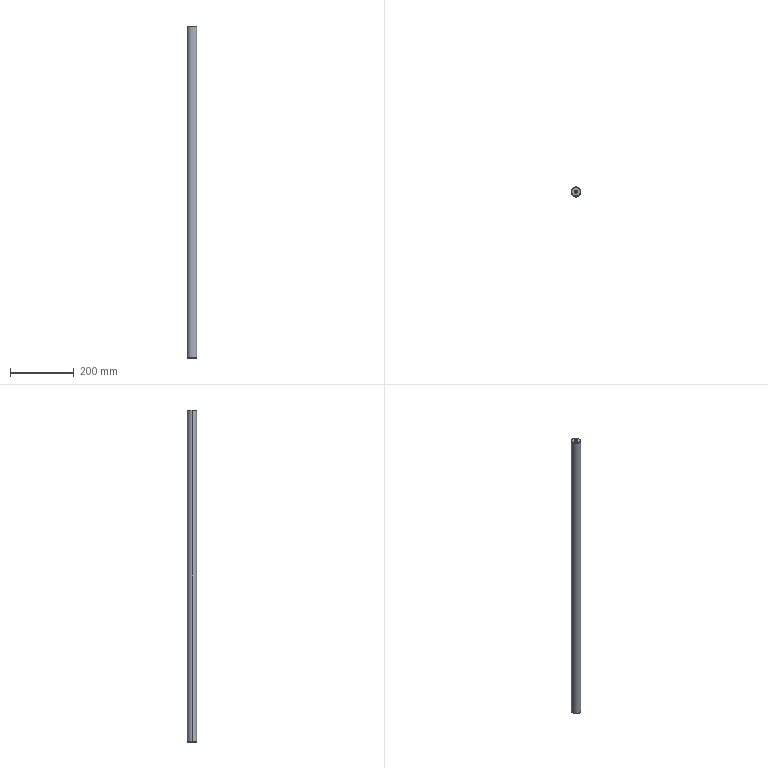Part | STEP file | Retracting rod | 1 solid | 18 faces | box 30 x 30 x 1045 mm | volume 737225 mm3 | cone 8 | cylinder 6 | plane 4 | commonest cylinder face diameters 6 x4 30 x2
STEP:
#1=CARTESIAN_POINT('',(-15.,0.,1043.));
#2=VERTEX_POINT('',#1);
#3=CARTESIAN_POINT('',(15.,0.,1043.));
#4=VERTEX_POINT('',#3);
#5=CARTESIAN_POINT('',(0.,0.,1043.));
#6=DIRECTION('',(0.,0.,-1.));
#7=DIRECTION('',(-1.,0.,0.));
#8=AXIS2_PLACEMENT_3D('',#5,#6,#7);
#9=CIRCLE('',#8,15.);
#10=EDGE_CURVE('',#2,#4,#9,.T.);
#11=ORIENTED_EDGE('',*,*,#10,.T.);
#12=CARTESIAN_POINT('',(15.,0.,2.));
#13=VERTEX_POINT('',#12);
#14=CARTESIAN_POINT('',(15.,0.,1045.));
#15=DIRECTION('',(0.,0.,-1.));
#16=VECTOR('',#15,1000.);
#17=LINE('',#14,#16);
#18=EDGE_CURVE('',#4,#13,#17,.T.);
#19=ORIENTED_EDGE('',*,*,#18,.T.);
#20=CARTESIAN_POINT('',(-15.,0.,2.));
#21=VERTEX_POINT('',#20);
#22=CARTESIAN_POINT('',(0.,0.,2.));
#23=DIRECTION('',(0.,0.,1.));
#24=DIRECTION('',(-1.,0.,0.));
#25=AXIS2_PLACEMENT_3D('',#22,#23,#24);
#26=CIRCLE('',#25,15.);
#27=EDGE_CURVE('',#13,#21,#26,.T.);
#28=ORIENTED_EDGE('',*,*,#27,.T.);
#29=CARTESIAN_POINT('',(-15.,0.,1045.));
#30=DIRECTION('',(0.,0.,-1.));
#31=VECTOR('',#30,1000.);
#32=LINE('',#29,#31);
#33=EDGE_CURVE('',#2,#21,#32,.T.);
#34=ORIENTED_EDGE('',*,*,#33,.F.);
#35=EDGE_LOOP('',(#11,#19,#28,#34));
#36=FACE_OUTER_BOUND('',#35,.T.);
#37=CARTESIAN_POINT('',(0.,0.,1045.));
#38=DIRECTION('',(0.,0.,-1.));
#39=DIRECTION('',(-1.,0.,0.));
#40=AXIS2_PLACEMENT_3D('',#37,#38,#39);
#41=CYLINDRICAL_SURFACE('',#40,15.);
#42=ADVANCED_FACE('',(#36),#41,.T.);
#43=CARTESIAN_POINT('',(13.,0.,0.));
#44=VERTEX_POINT('',#43);
#45=CARTESIAN_POINT('',(-13.,0.,0.));
#46=VERTEX_POINT('',#45);
#47=CARTESIAN_POINT('',(0.,0.,0.));
#48=DIRECTION('',(0.,0.,1.));
#49=DIRECTION('',(1.,0.,0.));
#50=AXIS2_PLACEMENT_3D('',#47,#48,#49);
#51=CIRCLE('',#50,13.);
#52=EDGE_CURVE('',#44,#46,#51,.T.);
#53=ORIENTED_EDGE('',*,*,#52,.T.);
#54=CARTESIAN_POINT('',(-15.,0.,2.));
#55=DIRECTION('',(-0.7071,0.,0.7071));
#56=VECTOR('',#55,1000.);
#57=LINE('',#54,#56);
#58=EDGE_CURVE('',#46,#21,#57,.T.);
#59=ORIENTED_EDGE('',*,*,#58,.T.);
#60=ORIENTED_EDGE('',*,*,#27,.F.);
#61=CARTESIAN_POINT('',(15.,0.,2.));
#62=DIRECTION('',(0.7071,0.,0.7071));
#63=VECTOR('',#62,1000.);
#64=LINE('',#61,#63);
#65=EDGE_CURVE('',#44,#13,#64,.T.);
#66=ORIENTED_EDGE('',*,*,#65,.F.);
#67=EDGE_LOOP('',(#53,#59,#60,#66));
#68=FACE_OUTER_BOUND('',#67,.T.);
#69=CARTESIAN_POINT('',(0.,0.,2.));
#70=DIRECTION('',(0.,0.,1.));
#71=DIRECTION('',(1.,0.,0.));
#72=AXIS2_PLACEMENT_3D('',#69,#70,#71);
#73=CONICAL_SURFACE('',#72,15.,0.7854);
#74=ADVANCED_FACE('',(#68),#73,.T.);
#75=CARTESIAN_POINT('',(-13.,0.,1045.));
#76=VERTEX_POINT('',#75);
#77=CARTESIAN_POINT('',(13.,0.,1045.));
#78=VERTEX_POINT('',#77);
#79=CARTESIAN_POINT('',(0.,0.,1045.));
#80=DIRECTION('',(0.,0.,-1.));
#81=DIRECTION('',(-1.,0.,0.));
#82=AXIS2_PLACEMENT_3D('',#79,#80,#81);
#83=CIRCLE('',#82,13.);
#84=EDGE_CURVE('',#76,#78,#83,.T.);
#85=ORIENTED_EDGE('',*,*,#84,.T.);
#86=CARTESIAN_POINT('',(15.,0.,1043.));
#87=DIRECTION('',(0.7071,0.,-0.7071));
#88=VECTOR('',#87,1000.);
#89=LINE('',#86,#88);
#90=EDGE_CURVE('',#78,#4,#89,.T.);
#91=ORIENTED_EDGE('',*,*,#90,.T.);
#92=ORIENTED_EDGE('',*,*,#10,.F.);
#93=CARTESIAN_POINT('',(-15.,0.,1043.));
#94=DIRECTION('',(-0.7071,0.,-0.7071));
#95=VECTOR('',#94,1000.);
#96=LINE('',#93,#95);
#97=EDGE_CURVE('',#76,#2,#96,.T.);
#98=ORIENTED_EDGE('',*,*,#97,.F.);
#99=EDGE_LOOP('',(#85,#91,#92,#98));
#100=FACE_OUTER_BOUND('',#99,.T.);
#101=CARTESIAN_POINT('',(0.,0.,1043.));
#102=DIRECTION('',(0.,0.,-1.));
#103=DIRECTION('',(-1.,0.,0.));
#104=AXIS2_PLACEMENT_3D('',#101,#102,#103);
#105=CONICAL_SURFACE('',#104,15.,0.7854);
#106=ADVANCED_FACE('',(#100),#105,.T.);
#107=CARTESIAN_POINT('',(3.,0.,2.));
#108=VERTEX_POINT('',#107);
#109=CARTESIAN_POINT('',(-3.,0.,2.));
#110=VERTEX_POINT('',#109);
#111=CARTESIAN_POINT('',(0.,0.,2.));
#112=DIRECTION('',(0.,0.,-1.));
#113=DIRECTION('',(-1.,0.,0.));
#114=AXIS2_PLACEMENT_3D('',#111,#112,#113);
#115=CIRCLE('',#114,3.);
#116=EDGE_CURVE('',#108,#110,#115,.T.);
#117=ORIENTED_EDGE('',*,*,#116,.F.);
#118=CARTESIAN_POINT('',(5.,0.,0.));
#119=VERTEX_POINT('',#118);
#120=CARTESIAN_POINT('',(5.,0.,0.));
#121=DIRECTION('',(0.7071,0.,-0.7071));
#122=VECTOR('',#121,1000.);
#123=LINE('',#120,#122);
#124=EDGE_CURVE('',#108,#119,#123,.T.);
#125=ORIENTED_EDGE('',*,*,#124,.T.);
#126=CARTESIAN_POINT('',(-5.,0.,0.));
#127=VERTEX_POINT('',#126);
#128=CARTESIAN_POINT('',(0.,0.,0.));
#129=DIRECTION('',(0.,0.,-1.));
#130=DIRECTION('',(-1.,0.,0.));
#131=AXIS2_PLACEMENT_3D('',#128,#129,#130);
#132=CIRCLE('',#131,5.);
#133=EDGE_CURVE('',#119,#127,#132,.T.);
#134=ORIENTED_EDGE('',*,*,#133,.T.);
#135=CARTESIAN_POINT('',(-5.,0.,0.));
#136=DIRECTION('',(-0.7071,0.,-0.7071));
#137=VECTOR('',#136,1000.);
#138=LINE('',#135,#137);
#139=EDGE_CURVE('',#110,#127,#138,.T.);
#140=ORIENTED_EDGE('',*,*,#139,.F.);
#141=EDGE_LOOP('',(#117,#125,#134,#140));
#142=FACE_OUTER_BOUND('',#141,.T.);
#143=CARTESIAN_POINT('',(0.,0.,0.));
#144=DIRECTION('',(0.,0.,-1.));
#145=DIRECTION('',(-1.,0.,0.));
#146=AXIS2_PLACEMENT_3D('',#143,#144,#145);
#147=CONICAL_SURFACE('',#146,5.,0.7854);
#148=ADVANCED_FACE('',(#142),#147,.F.);
#149=CARTESIAN_POINT('',(-3.,0.,1043.));
#150=VERTEX_POINT('',#149);
#151=CARTESIAN_POINT('',(3.,0.,1043.));
#152=VERTEX_POINT('',#151);
#153=CARTESIAN_POINT('',(0.,0.,1043.));
#154=DIRECTION('',(0.,0.,1.));
#155=DIRECTION('',(1.,0.,0.));
#156=AXIS2_PLACEMENT_3D('',#153,#154,#155);
#157=CIRCLE('',#156,3.);
#158=EDGE_CURVE('',#150,#152,#157,.T.);
#159=ORIENTED_EDGE('',*,*,#158,.F.);
#160=CARTESIAN_POINT('',(-5.,0.,1045.));
#161=VERTEX_POINT('',#160);
#162=CARTESIAN_POINT('',(-5.,0.,1045.));
#163=DIRECTION('',(-0.7071,0.,0.7071));
#164=VECTOR('',#163,1000.);
#165=LINE('',#162,#164);
#166=EDGE_CURVE('',#150,#161,#165,.T.);
#167=ORIENTED_EDGE('',*,*,#166,.T.);
#168=CARTESIAN_POINT('',(5.,0.,1045.));
#169=VERTEX_POINT('',#168);
#170=CARTESIAN_POINT('',(0.,0.,1045.));
#171=DIRECTION('',(0.,0.,-1.));
#172=DIRECTION('',(1.,0.,0.));
#173=AXIS2_PLACEMENT_3D('',#170,#171,#172);
#174=CIRCLE('',#173,5.);
#175=EDGE_CURVE('',#169,#161,#174,.T.);
#176=ORIENTED_EDGE('',*,*,#175,.F.);
#177=CARTESIAN_POINT('',(5.,0.,1045.));
#178=DIRECTION('',(0.7071,0.,0.7071));
#179=VECTOR('',#178,1000.);
#180=LINE('',#177,#179);
#181=EDGE_CURVE('',#152,#169,#180,.T.);
#182=ORIENTED_EDGE('',*,*,#181,.F.);
#183=EDGE_LOOP('',(#159,#167,#176,#182));
#184=FACE_OUTER_BOUND('',#183,.T.);
#185=CARTESIAN_POINT('',(0.,0.,1045.));
#186=DIRECTION('',(0.,0.,1.));
#187=DIRECTION('',(1.,0.,0.));
#188=AXIS2_PLACEMENT_3D('',#185,#186,#187);
#189=CONICAL_SURFACE('',#188,5.,0.7854);
#190=ADVANCED_FACE('',(#184),#189,.F.);
#191=CARTESIAN_POINT('',(3.,0.,20.));
#192=VERTEX_POINT('',#191);
#193=CARTESIAN_POINT('',(-3.,0.,20.));
#194=VERTEX_POINT('',#193);
#195=CARTESIAN_POINT('',(0.,0.,20.));
#196=DIRECTION('',(0.,0.,-1.));
#197=DIRECTION('',(-1.,0.,0.));
#198=AXIS2_PLACEMENT_3D('',#195,#196,#197);
#199=CIRCLE('',#198,3.);
#200=EDGE_CURVE('',#192,#194,#199,.T.);
#201=ORIENTED_EDGE('',*,*,#200,.F.);
#202=CARTESIAN_POINT('',(3.,0.,20.));
#203=DIRECTION('',(0.,0.,-1.));
#204=VECTOR('',#203,1000.);
#205=LINE('',#202,#204);
#206=EDGE_CURVE('',#192,#108,#205,.T.);
#207=ORIENTED_EDGE('',*,*,#206,.T.);
#208=ORIENTED_EDGE('',*,*,#116,.T.);
#209=CARTESIAN_POINT('',(-3.,0.,20.));
#210=DIRECTION('',(0.,0.,-1.));
#211=VECTOR('',#210,1000.);
#212=LINE('',#209,#211);
#213=EDGE_CURVE('',#194,#110,#212,.T.);
#214=ORIENTED_EDGE('',*,*,#213,.F.);
#215=EDGE_LOOP('',(#201,#207,#208,#214));
#216=FACE_OUTER_BOUND('',#215,.T.);
#217=CARTESIAN_POINT('',(0.,0.,20.));
#218=DIRECTION('',(0.,0.,-1.));
#219=DIRECTION('',(-1.,0.,0.));
#220=AXIS2_PLACEMENT_3D('',#217,#218,#219);
#221=CYLINDRICAL_SURFACE('',#220,3.);
#222=ADVANCED_FACE('',(#216),#221,.F.);
#223=CARTESIAN_POINT('',(-3.,0.,1030.));
#224=VERTEX_POINT('',#223);
#225=CARTESIAN_POINT('',(3.,0.,1030.));
#226=VERTEX_POINT('',#225);
#227=CARTESIAN_POINT('',(0.,0.,1030.));
#228=DIRECTION('',(0.,0.,1.));
#229=DIRECTION('',(1.,0.,0.));
#230=AXIS2_PLACEMENT_3D('',#227,#228,#229);
#231=CIRCLE('',#230,3.);
#232=EDGE_CURVE('',#224,#226,#231,.T.);
#233=ORIENTED_EDGE('',*,*,#232,.F.);
#234=CARTESIAN_POINT('',(-3.,0.,1030.));
#235=DIRECTION('',(0.,0.,1.));
#236=VECTOR('',#235,1000.);
#237=LINE('',#234,#236);
#238=EDGE_CURVE('',#224,#150,#237,.T.);
#239=ORIENTED_EDGE('',*,*,#238,.T.);
#240=ORIENTED_EDGE('',*,*,#158,.T.);
#241=CARTESIAN_POINT('',(3.,0.,1030.));
#242=DIRECTION('',(0.,0.,1.));
#243=VECTOR('',#242,1000.);
#244=LINE('',#241,#243);
#245=EDGE_CURVE('',#226,#152,#244,.T.);
#246=ORIENTED_EDGE('',*,*,#245,.F.);
#247=EDGE_LOOP('',(#233,#239,#240,#246));
#248=FACE_OUTER_BOUND('',#247,.T.);
#249=CARTESIAN_POINT('',(0.,0.,1030.));
#250=DIRECTION('',(0.,0.,1.));
#251=DIRECTION('',(1.,0.,0.));
#252=AXIS2_PLACEMENT_3D('',#249,#250,#251);
#253=CYLINDRICAL_SURFACE('',#252,3.);
#254=ADVANCED_FACE('',(#248),#253,.F.);
#255=ORIENTED_EDGE('',*,*,#18,.F.);
#256=CARTESIAN_POINT('',(0.,0.,1043.));
#257=DIRECTION('',(0.,0.,-1.));
#258=DIRECTION('',(-1.,0.,0.));
#259=AXIS2_PLACEMENT_3D('',#256,#257,#258);
#260=CIRCLE('',#259,15.);
#261=EDGE_CURVE('',#4,#2,#260,.T.);
#262=ORIENTED_EDGE('',*,*,#261,.T.);
#263=ORIENTED_EDGE('',*,*,#33,.T.);
#264=CARTESIAN_POINT('',(0.,0.,2.));
#265=DIRECTION('',(0.,0.,1.));
#266=DIRECTION('',(-1.,0.,0.));
#267=AXIS2_PLACEMENT_3D('',#264,#265,#266);
#268=CIRCLE('',#267,15.);
#269=EDGE_CURVE('',#21,#13,#268,.T.);
#270=ORIENTED_EDGE('',*,*,#269,.T.);
#271=EDGE_LOOP('',(#255,#262,#263,#270));
#272=FACE_OUTER_BOUND('',#271,.T.);
#273=CARTESIAN_POINT('',(0.,0.,1045.));
#274=DIRECTION('',(0.,0.,-1.));
#275=DIRECTION('',(-1.,0.,0.));
#276=AXIS2_PLACEMENT_3D('',#273,#274,#275);
#277=CYLINDRICAL_SURFACE('',#276,15.);
#278=ADVANCED_FACE('',(#272),#277,.T.);
#279=ORIENTED_EDGE('',*,*,#58,.F.);
#280=CARTESIAN_POINT('',(0.,0.,0.));
#281=DIRECTION('',(0.,0.,1.));
#282=DIRECTION('',(1.,0.,0.));
#283=AXIS2_PLACEMENT_3D('',#280,#281,#282);
#284=CIRCLE('',#283,13.);
#285=EDGE_CURVE('',#46,#44,#284,.T.);
#286=ORIENTED_EDGE('',*,*,#285,.T.);
#287=ORIENTED_EDGE('',*,*,#65,.T.);
#288=ORIENTED_EDGE('',*,*,#269,.F.);
#289=EDGE_LOOP('',(#279,#286,#287,#288));
#290=FACE_OUTER_BOUND('',#289,.T.);
#291=CARTESIAN_POINT('',(0.,0.,2.));
#292=DIRECTION('',(0.,0.,1.));
#293=DIRECTION('',(1.,0.,0.));
#294=AXIS2_PLACEMENT_3D('',#291,#292,#293);
#295=CONICAL_SURFACE('',#294,15.,0.7854);
#296=ADVANCED_FACE('',(#290),#295,.T.);
#297=ORIENTED_EDGE('',*,*,#90,.F.);
#298=CARTESIAN_POINT('',(0.,0.,1045.));
#299=DIRECTION('',(0.,0.,-1.));
#300=DIRECTION('',(-1.,0.,0.));
#301=AXIS2_PLACEMENT_3D('',#298,#299,#300);
#302=CIRCLE('',#301,13.);
#303=EDGE_CURVE('',#78,#76,#302,.T.);
#304=ORIENTED_EDGE('',*,*,#303,.T.);
#305=ORIENTED_EDGE('',*,*,#97,.T.);
#306=ORIENTED_EDGE('',*,*,#261,.F.);
#307=EDGE_LOOP('',(#297,#304,#305,#306));
#308=FACE_OUTER_BOUND('',#307,.T.);
#309=CARTESIAN_POINT('',(0.,0.,1043.));
#310=DIRECTION('',(0.,0.,-1.));
#311=DIRECTION('',(-1.,0.,0.));
#312=AXIS2_PLACEMENT_3D('',#309,#310,#311);
#313=CONICAL_SURFACE('',#312,15.,0.7854);
#314=ADVANCED_FACE('',(#308),#313,.T.);
#315=ORIENTED_EDGE('',*,*,#52,.F.);
#316=ORIENTED_EDGE('',*,*,#285,.F.);
#317=EDGE_LOOP('',(#315,#316));
#318=FACE_OUTER_BOUND('',#317,.T.);
#319=CARTESIAN_POINT('',(0.,0.,0.));
#320=DIRECTION('',(0.,0.,-1.));
#321=DIRECTION('',(-1.,0.,0.));
#322=AXIS2_PLACEMENT_3D('',#319,#320,#321);
#323=CIRCLE('',#322,5.);
#324=EDGE_CURVE('',#127,#119,#323,.T.);
#325=ORIENTED_EDGE('',*,*,#324,.F.);
#326=ORIENTED_EDGE('',*,*,#133,.F.);
#327=EDGE_LOOP('',(#325,#326));
#328=FACE_BOUND('',#327,.T.);
#329=CARTESIAN_POINT('',(0.,0.,0.));
#330=DIRECTION('',(0.,0.,1.));
#331=DIRECTION('',(1.,0.,0.));
#332=AXIS2_PLACEMENT_3D('',#329,#330,#331);
#333=PLANE('',#332);
#334=ADVANCED_FACE('',(#318,#328),#333,.F.);
#335=ORIENTED_EDGE('',*,*,#84,.F.);
#336=ORIENTED_EDGE('',*,*,#303,.F.);
#337=EDGE_LOOP('',(#335,#336));
#338=FACE_OUTER_BOUND('',#337,.T.);
#339=ORIENTED_EDGE('',*,*,#175,.T.);
#340=CARTESIAN_POINT('',(0.,0.,1045.));
#341=DIRECTION('',(0.,0.,-1.));
#342=DIRECTION('',(1.,0.,0.));
#343=AXIS2_PLACEMENT_3D('',#340,#341,#342);
#344=CIRCLE('',#343,5.);
#345=EDGE_CURVE('',#161,#169,#344,.T.);
#346=ORIENTED_EDGE('',*,*,#345,.T.);
#347=EDGE_LOOP('',(#339,#346));
#348=FACE_BOUND('',#347,.T.);
#349=CARTESIAN_POINT('',(0.,0.,1045.));
#350=DIRECTION('',(0.,0.,1.));
#351=DIRECTION('',(1.,0.,0.));
#352=AXIS2_PLACEMENT_3D('',#349,#350,#351);
#353=PLANE('',#352);
#354=ADVANCED_FACE('',(#338,#348),#353,.T.);
#355=ORIENTED_EDGE('',*,*,#124,.F.);
#356=CARTESIAN_POINT('',(0.,0.,2.));
#357=DIRECTION('',(0.,0.,-1.));
#358=DIRECTION('',(-1.,0.,0.));
#359=AXIS2_PLACEMENT_3D('',#356,#357,#358);
#360=CIRCLE('',#359,3.);
#361=EDGE_CURVE('',#110,#108,#360,.T.);
#362=ORIENTED_EDGE('',*,*,#361,.F.);
#363=ORIENTED_EDGE('',*,*,#139,.T.);
#364=ORIENTED_EDGE('',*,*,#324,.T.);
#365=EDGE_LOOP('',(#355,#362,#363,#364));
#366=FACE_OUTER_BOUND('',#365,.T.);
#367=CARTESIAN_POINT('',(0.,0.,0.));
#368=DIRECTION('',(0.,0.,-1.));
#369=DIRECTION('',(-1.,0.,0.));
#370=AXIS2_PLACEMENT_3D('',#367,#368,#369);
#371=CONICAL_SURFACE('',#370,5.,0.7854);
#372=ADVANCED_FACE('',(#366),#371,.F.);
#373=ORIENTED_EDGE('',*,*,#166,.F.);
#374=CARTESIAN_POINT('',(0.,0.,1043.));
#375=DIRECTION('',(0.,0.,1.));
#376=DIRECTION('',(1.,0.,0.));
#377=AXIS2_PLACEMENT_3D('',#374,#375,#376);
#378=CIRCLE('',#377,3.);
#379=EDGE_CURVE('',#152,#150,#378,.T.);
#380=ORIENTED_EDGE('',*,*,#379,.F.);
#381=ORIENTED_EDGE('',*,*,#181,.T.);
#382=ORIENTED_EDGE('',*,*,#345,.F.);
#383=EDGE_LOOP('',(#373,#380,#381,#382));
#384=FACE_OUTER_BOUND('',#383,.T.);
#385=CARTESIAN_POINT('',(0.,0.,1045.));
#386=DIRECTION('',(0.,0.,1.));
#387=DIRECTION('',(1.,0.,0.));
#388=AXIS2_PLACEMENT_3D('',#385,#386,#387);
#389=CONICAL_SURFACE('',#388,5.,0.7854);
#390=ADVANCED_FACE('',(#384),#389,.F.);
#391=ORIENTED_EDGE('',*,*,#206,.F.);
#392=CARTESIAN_POINT('',(0.,0.,20.));
#393=DIRECTION('',(0.,0.,-1.));
#394=DIRECTION('',(-1.,0.,0.));
#395=AXIS2_PLACEMENT_3D('',#392,#393,#394);
#396=CIRCLE('',#395,3.);
#397=EDGE_CURVE('',#194,#192,#396,.T.);
#398=ORIENTED_EDGE('',*,*,#397,.F.);
#399=ORIENTED_EDGE('',*,*,#213,.T.);
#400=ORIENTED_EDGE('',*,*,#361,.T.);
#401=EDGE_LOOP('',(#391,#398,#399,#400));
#402=FACE_OUTER_BOUND('',#401,.T.);
#403=CARTESIAN_POINT('',(0.,0.,20.));
#404=DIRECTION('',(0.,0.,-1.));
#405=DIRECTION('',(-1.,0.,0.));
#406=AXIS2_PLACEMENT_3D('',#403,#404,#405);
#407=CYLINDRICAL_SURFACE('',#406,3.);
#408=ADVANCED_FACE('',(#402),#407,.F.);
#409=ORIENTED_EDGE('',*,*,#238,.F.);
#410=CARTESIAN_POINT('',(0.,0.,1030.));
#411=DIRECTION('',(0.,0.,1.));
#412=DIRECTION('',(1.,0.,0.));
#413=AXIS2_PLACEMENT_3D('',#410,#411,#412);
#414=CIRCLE('',#413,3.);
#415=EDGE_CURVE('',#226,#224,#414,.T.);
#416=ORIENTED_EDGE('',*,*,#415,.F.);
#417=ORIENTED_EDGE('',*,*,#245,.T.);
#418=ORIENTED_EDGE('',*,*,#379,.T.);
#419=EDGE_LOOP('',(#409,#416,#417,#418));
#420=FACE_OUTER_BOUND('',#419,.T.);
#421=CARTESIAN_POINT('',(0.,0.,1030.));
#422=DIRECTION('',(0.,0.,1.));
#423=DIRECTION('',(1.,0.,0.));
#424=AXIS2_PLACEMENT_3D('',#421,#422,#423);
#425=CYLINDRICAL_SURFACE('',#424,3.);
#426=ADVANCED_FACE('',(#420),#425,.F.);
#427=ORIENTED_EDGE('',*,*,#397,.T.);
#428=ORIENTED_EDGE('',*,*,#200,.T.);
#429=EDGE_LOOP('',(#427,#428));
#430=FACE_OUTER_BOUND('',#429,.T.);
#431=CARTESIAN_POINT('',(0.,0.,20.));
#432=DIRECTION('',(0.,0.,-1.));
#433=DIRECTION('',(-1.,0.,0.));
#434=AXIS2_PLACEMENT_3D('',#431,#432,#433);
#435=PLANE('',#434);
#436=ADVANCED_FACE('',(#430),#435,.T.);
#437=ORIENTED_EDGE('',*,*,#415,.T.);
#438=ORIENTED_EDGE('',*,*,#232,.T.);
#439=EDGE_LOOP('',(#437,#438));
#440=FACE_OUTER_BOUND('',#439,.T.);
#441=CARTESIAN_POINT('',(0.,0.,1030.));
#442=DIRECTION('',(0.,0.,1.));
#443=DIRECTION('',(1.,0.,0.));
#444=AXIS2_PLACEMENT_3D('',#441,#442,#443);
#445=PLANE('',#444);
#446=ADVANCED_FACE('',(#440),#445,.T.);
#447=CLOSED_SHELL('',(#42,#74,#106,#148,#190,#222,#254,#278,#296,#314,#334,#354,#372,#390,#408,#426,#436,#446));
#448=MANIFOLD_SOLID_BREP('',#447);
#449=CARTESIAN_POINT('',(0.,0.,0.));
#450=DIRECTION('',(0.,0.,1.));
#451=DIRECTION('',(1.,0.,0.));
#452=AXIS2_PLACEMENT_3D('',#449,#450,#451);
#453=(LENGTH_UNIT()NAMED_UNIT(*)SI_UNIT(.MILLI.,.METRE.));
#454=UNCERTAINTY_MEASURE_WITH_UNIT(LENGTH_MEASURE(0.00001),#453,'','');
#455=(NAMED_UNIT(*)PLANE_ANGLE_UNIT()SI_UNIT($,.RADIAN.));
#456=(NAMED_UNIT(*)SI_UNIT($,.STERADIAN.)SOLID_ANGLE_UNIT());
#457=(GEOMETRIC_REPRESENTATION_CONTEXT(3)GLOBAL_UNCERTAINTY_ASSIGNED_CONTEXT((#454))GLOBAL_UNIT_ASSIGNED_CONTEXT((#453,#455,#456))REPRESENTATION_CONTEXT('',''));
#458=ADVANCED_BREP_SHAPE_REPRESENTATION('',(#448,#452),#457);